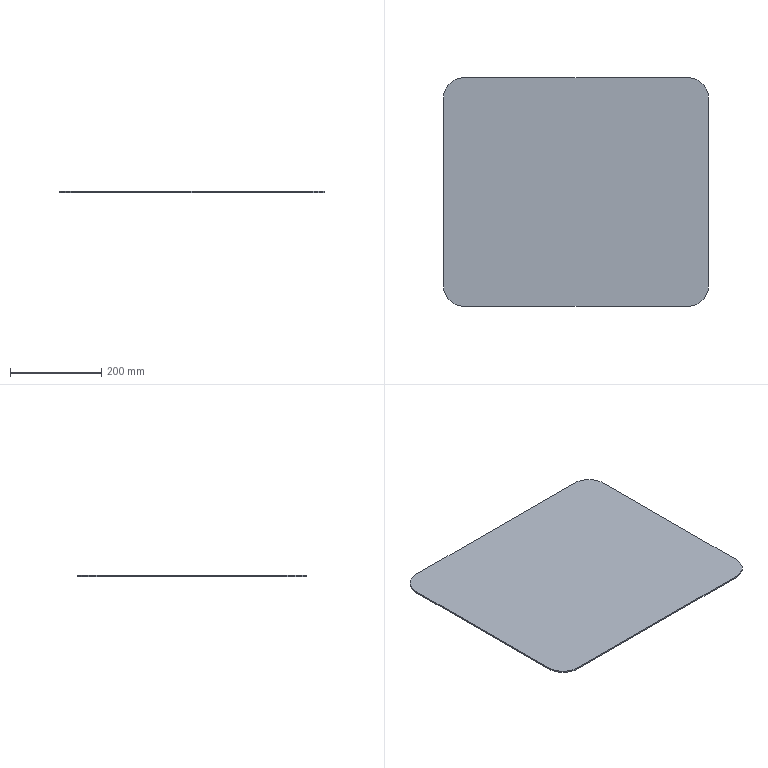Part | STEP file | Glass plate | 1 solid | 10 faces | box 580 x 500 x 3 mm | volume 864785 mm3 | plane 6 | cylinder 4 | commonest cylinder face diameters 90 x4
STEP:
#1=CARTESIAN_POINT('',(0.,0.,0.));
#2=DIRECTION('',(0.,0.,1.));
#3=DIRECTION('',(1.,0.,0.));
#4=AXIS2_PLACEMENT_3D('',#1,#2,#3);
#5=CARTESIAN_POINT('',(245.,-250.,0.));
#6=VERTEX_POINT('',#5);
#7=CARTESIAN_POINT('',(290.,-205.,0.));
#8=VERTEX_POINT('',#7);
#9=CARTESIAN_POINT('',(245.,-205.,0.));
#10=DIRECTION('',(0.,0.,1.));
#11=DIRECTION('',(1.,0.,0.));
#12=AXIS2_PLACEMENT_3D('',#9,#10,#11);
#13=CIRCLE('',#12,45.);
#14=CARTESIAN_POINT('',(0.,0.,0.));
#15=DIRECTION('',(0.,0.,1.));
#16=DIRECTION('',(1.,0.,0.));
#17=AXIS2_PLACEMENT_3D('',#14,#15,#16);
#18=PLANE('',#17);
#19=CARTESIAN_POINT('',(245.,-205.));
#20=DIRECTION('',(1.,0.));
#21=AXIS2_PLACEMENT_2D('',#19,#20);
#22=CIRCLE('',#21,45.);
#23=(GEOMETRIC_REPRESENTATION_CONTEXT(2)PARAMETRIC_REPRESENTATION_CONTEXT()REPRESENTATION_CONTEXT('',''));
#24=DEFINITIONAL_REPRESENTATION('',(#22),#23);
#25=PCURVE('',#18,#24);
#26=CARTESIAN_POINT('',(245.,-205.,-2.));
#27=DIRECTION('',(0.,0.,1.));
#28=DIRECTION('',(1.,0.,0.));
#29=AXIS2_PLACEMENT_3D('',#26,#27,#28);
#30=CYLINDRICAL_SURFACE('',#29,45.);
#31=CARTESIAN_POINT('',(0.,2.));
#32=DIRECTION('',(1.,0.));
#33=VECTOR('',#32,1.);
#34=LINE('',#31,#33);
#35=(GEOMETRIC_REPRESENTATION_CONTEXT(2)PARAMETRIC_REPRESENTATION_CONTEXT()REPRESENTATION_CONTEXT('',''));
#36=DEFINITIONAL_REPRESENTATION('',(#34),#35);
#37=PCURVE('',#30,#36);
#38=SURFACE_CURVE('',#13,(#25,#37),.PCURVE_S1.);
#39=EDGE_CURVE('',#6,#8,#38,.T.);
#40=ORIENTED_EDGE('',*,*,#39,.F.);
#41=CARTESIAN_POINT('',(-245.,-250.,0.));
#42=VERTEX_POINT('',#41);
#43=CARTESIAN_POINT('',(0.,-250.,0.));
#44=DIRECTION('',(1.,0.,0.));
#45=VECTOR('',#44,1.);
#46=LINE('',#43,#45);
#47=CARTESIAN_POINT('',(0.,-250.));
#48=DIRECTION('',(1.,0.));
#49=VECTOR('',#48,1.);
#50=LINE('',#47,#49);
#51=(GEOMETRIC_REPRESENTATION_CONTEXT(2)PARAMETRIC_REPRESENTATION_CONTEXT()REPRESENTATION_CONTEXT('',''));
#52=DEFINITIONAL_REPRESENTATION('',(#50),#51);
#53=PCURVE('',#18,#52);
#54=CARTESIAN_POINT('',(-245.,-250.,-2.));
#55=DIRECTION('',(0.,-1.,0.));
#56=DIRECTION('',(1.,0.,0.));
#57=AXIS2_PLACEMENT_3D('',#54,#55,#56);
#58=PLANE('',#57);
#59=CARTESIAN_POINT('',(245.,2.));
#60=DIRECTION('',(1.,0.));
#61=VECTOR('',#60,1.);
#62=LINE('',#59,#61);
#63=(GEOMETRIC_REPRESENTATION_CONTEXT(2)PARAMETRIC_REPRESENTATION_CONTEXT()REPRESENTATION_CONTEXT('',''));
#64=DEFINITIONAL_REPRESENTATION('',(#62),#63);
#65=PCURVE('',#58,#64);
#66=SURFACE_CURVE('',#46,(#53,#65),.PCURVE_S1.);
#67=EDGE_CURVE('',#42,#6,#66,.T.);
#68=ORIENTED_EDGE('',*,*,#67,.F.);
#69=CARTESIAN_POINT('',(-290.,-205.,0.));
#70=VERTEX_POINT('',#69);
#71=CARTESIAN_POINT('',(-245.,-205.,0.));
#72=DIRECTION('',(0.,0.,1.));
#73=DIRECTION('',(1.,0.,0.));
#74=AXIS2_PLACEMENT_3D('',#71,#72,#73);
#75=CIRCLE('',#74,45.);
#76=CARTESIAN_POINT('',(-245.,-205.));
#77=DIRECTION('',(1.,0.));
#78=AXIS2_PLACEMENT_2D('',#76,#77);
#79=CIRCLE('',#78,45.);
#80=(GEOMETRIC_REPRESENTATION_CONTEXT(2)PARAMETRIC_REPRESENTATION_CONTEXT()REPRESENTATION_CONTEXT('',''));
#81=DEFINITIONAL_REPRESENTATION('',(#79),#80);
#82=PCURVE('',#18,#81);
#83=CARTESIAN_POINT('',(-245.,-205.,-2.));
#84=DIRECTION('',(0.,0.,1.));
#85=DIRECTION('',(1.,0.,0.));
#86=AXIS2_PLACEMENT_3D('',#83,#84,#85);
#87=CYLINDRICAL_SURFACE('',#86,45.);
#88=CARTESIAN_POINT('',(0.,2.));
#89=DIRECTION('',(1.,0.));
#90=VECTOR('',#89,1.);
#91=LINE('',#88,#90);
#92=(GEOMETRIC_REPRESENTATION_CONTEXT(2)PARAMETRIC_REPRESENTATION_CONTEXT()REPRESENTATION_CONTEXT('',''));
#93=DEFINITIONAL_REPRESENTATION('',(#91),#92);
#94=PCURVE('',#87,#93);
#95=SURFACE_CURVE('',#75,(#82,#94),.PCURVE_S1.);
#96=EDGE_CURVE('',#70,#42,#95,.T.);
#97=ORIENTED_EDGE('',*,*,#96,.F.);
#98=CARTESIAN_POINT('',(-290.,205.,0.));
#99=VERTEX_POINT('',#98);
#100=CARTESIAN_POINT('',(-290.,0.,0.));
#101=DIRECTION('',(0.,-1.,0.));
#102=VECTOR('',#101,1.);
#103=LINE('',#100,#102);
#104=CARTESIAN_POINT('',(-290.,0.));
#105=DIRECTION('',(0.,-1.));
#106=VECTOR('',#105,1.);
#107=LINE('',#104,#106);
#108=(GEOMETRIC_REPRESENTATION_CONTEXT(2)PARAMETRIC_REPRESENTATION_CONTEXT()REPRESENTATION_CONTEXT('',''));
#109=DEFINITIONAL_REPRESENTATION('',(#107),#108);
#110=PCURVE('',#18,#109);
#111=CARTESIAN_POINT('',(-290.,205.,-2.));
#112=DIRECTION('',(-1.,0.,0.));
#113=DIRECTION('',(0.,-1.,0.));
#114=AXIS2_PLACEMENT_3D('',#111,#112,#113);
#115=PLANE('',#114);
#116=CARTESIAN_POINT('',(205.,2.));
#117=DIRECTION('',(1.,0.));
#118=VECTOR('',#117,1.);
#119=LINE('',#116,#118);
#120=(GEOMETRIC_REPRESENTATION_CONTEXT(2)PARAMETRIC_REPRESENTATION_CONTEXT()REPRESENTATION_CONTEXT('',''));
#121=DEFINITIONAL_REPRESENTATION('',(#119),#120);
#122=PCURVE('',#115,#121);
#123=SURFACE_CURVE('',#103,(#110,#122),.PCURVE_S1.);
#124=EDGE_CURVE('',#99,#70,#123,.T.);
#125=ORIENTED_EDGE('',*,*,#124,.F.);
#126=CARTESIAN_POINT('',(-245.,250.,0.));
#127=VERTEX_POINT('',#126);
#128=CARTESIAN_POINT('',(-245.,205.,0.));
#129=DIRECTION('',(0.,0.,1.));
#130=DIRECTION('',(1.,0.,0.));
#131=AXIS2_PLACEMENT_3D('',#128,#129,#130);
#132=CIRCLE('',#131,45.);
#133=CARTESIAN_POINT('',(-245.,205.));
#134=DIRECTION('',(1.,0.));
#135=AXIS2_PLACEMENT_2D('',#133,#134);
#136=CIRCLE('',#135,45.);
#137=(GEOMETRIC_REPRESENTATION_CONTEXT(2)PARAMETRIC_REPRESENTATION_CONTEXT()REPRESENTATION_CONTEXT('',''));
#138=DEFINITIONAL_REPRESENTATION('',(#136),#137);
#139=PCURVE('',#18,#138);
#140=CARTESIAN_POINT('',(-245.,205.,-2.));
#141=DIRECTION('',(0.,0.,1.));
#142=DIRECTION('',(1.,0.,0.));
#143=AXIS2_PLACEMENT_3D('',#140,#141,#142);
#144=CYLINDRICAL_SURFACE('',#143,45.);
#145=CARTESIAN_POINT('',(0.,2.));
#146=DIRECTION('',(1.,0.));
#147=VECTOR('',#146,1.);
#148=LINE('',#145,#147);
#149=(GEOMETRIC_REPRESENTATION_CONTEXT(2)PARAMETRIC_REPRESENTATION_CONTEXT()REPRESENTATION_CONTEXT('',''));
#150=DEFINITIONAL_REPRESENTATION('',(#148),#149);
#151=PCURVE('',#144,#150);
#152=SURFACE_CURVE('',#132,(#139,#151),.PCURVE_S1.);
#153=EDGE_CURVE('',#127,#99,#152,.T.);
#154=ORIENTED_EDGE('',*,*,#153,.F.);
#155=CARTESIAN_POINT('',(245.,250.,0.));
#156=VERTEX_POINT('',#155);
#157=CARTESIAN_POINT('',(0.,250.,0.));
#158=DIRECTION('',(-1.,0.,0.));
#159=VECTOR('',#158,1.);
#160=LINE('',#157,#159);
#161=CARTESIAN_POINT('',(0.,250.));
#162=DIRECTION('',(-1.,0.));
#163=VECTOR('',#162,1.);
#164=LINE('',#161,#163);
#165=(GEOMETRIC_REPRESENTATION_CONTEXT(2)PARAMETRIC_REPRESENTATION_CONTEXT()REPRESENTATION_CONTEXT('',''));
#166=DEFINITIONAL_REPRESENTATION('',(#164),#165);
#167=PCURVE('',#18,#166);
#168=CARTESIAN_POINT('',(245.,250.,-2.));
#169=DIRECTION('',(0.,1.,0.));
#170=DIRECTION('',(-1.,0.,0.));
#171=AXIS2_PLACEMENT_3D('',#168,#169,#170);
#172=PLANE('',#171);
#173=CARTESIAN_POINT('',(245.,2.));
#174=DIRECTION('',(1.,0.));
#175=VECTOR('',#174,1.);
#176=LINE('',#173,#175);
#177=(GEOMETRIC_REPRESENTATION_CONTEXT(2)PARAMETRIC_REPRESENTATION_CONTEXT()REPRESENTATION_CONTEXT('',''));
#178=DEFINITIONAL_REPRESENTATION('',(#176),#177);
#179=PCURVE('',#172,#178);
#180=SURFACE_CURVE('',#160,(#167,#179),.PCURVE_S1.);
#181=EDGE_CURVE('',#156,#127,#180,.T.);
#182=ORIENTED_EDGE('',*,*,#181,.F.);
#183=CARTESIAN_POINT('',(290.,205.,0.));
#184=VERTEX_POINT('',#183);
#185=CARTESIAN_POINT('',(245.,205.,0.));
#186=DIRECTION('',(0.,0.,1.));
#187=DIRECTION('',(1.,0.,0.));
#188=AXIS2_PLACEMENT_3D('',#185,#186,#187);
#189=CIRCLE('',#188,45.);
#190=CARTESIAN_POINT('',(245.,205.));
#191=DIRECTION('',(1.,0.));
#192=AXIS2_PLACEMENT_2D('',#190,#191);
#193=CIRCLE('',#192,45.);
#194=(GEOMETRIC_REPRESENTATION_CONTEXT(2)PARAMETRIC_REPRESENTATION_CONTEXT()REPRESENTATION_CONTEXT('',''));
#195=DEFINITIONAL_REPRESENTATION('',(#193),#194);
#196=PCURVE('',#18,#195);
#197=CARTESIAN_POINT('',(245.,205.,-2.));
#198=DIRECTION('',(0.,0.,1.));
#199=DIRECTION('',(1.,0.,0.));
#200=AXIS2_PLACEMENT_3D('',#197,#198,#199);
#201=CYLINDRICAL_SURFACE('',#200,45.);
#202=CARTESIAN_POINT('',(0.,2.));
#203=DIRECTION('',(1.,0.));
#204=VECTOR('',#203,1.);
#205=LINE('',#202,#204);
#206=(GEOMETRIC_REPRESENTATION_CONTEXT(2)PARAMETRIC_REPRESENTATION_CONTEXT()REPRESENTATION_CONTEXT('',''));
#207=DEFINITIONAL_REPRESENTATION('',(#205),#206);
#208=PCURVE('',#201,#207);
#209=SURFACE_CURVE('',#189,(#196,#208),.PCURVE_S1.);
#210=EDGE_CURVE('',#184,#156,#209,.T.);
#211=ORIENTED_EDGE('',*,*,#210,.F.);
#212=CARTESIAN_POINT('',(290.,0.,0.));
#213=DIRECTION('',(0.,1.,0.));
#214=VECTOR('',#213,1.);
#215=LINE('',#212,#214);
#216=CARTESIAN_POINT('',(290.,0.));
#217=DIRECTION('',(0.,1.));
#218=VECTOR('',#217,1.);
#219=LINE('',#216,#218);
#220=(GEOMETRIC_REPRESENTATION_CONTEXT(2)PARAMETRIC_REPRESENTATION_CONTEXT()REPRESENTATION_CONTEXT('',''));
#221=DEFINITIONAL_REPRESENTATION('',(#219),#220);
#222=PCURVE('',#18,#221);
#223=CARTESIAN_POINT('',(290.,-205.,-2.));
#224=DIRECTION('',(1.,0.,0.));
#225=DIRECTION('',(0.,1.,0.));
#226=AXIS2_PLACEMENT_3D('',#223,#224,#225);
#227=PLANE('',#226);
#228=CARTESIAN_POINT('',(205.,2.));
#229=DIRECTION('',(1.,0.));
#230=VECTOR('',#229,1.);
#231=LINE('',#228,#230);
#232=(GEOMETRIC_REPRESENTATION_CONTEXT(2)PARAMETRIC_REPRESENTATION_CONTEXT()REPRESENTATION_CONTEXT('',''));
#233=DEFINITIONAL_REPRESENTATION('',(#231),#232);
#234=PCURVE('',#227,#233);
#235=SURFACE_CURVE('',#215,(#222,#234),.PCURVE_S1.);
#236=EDGE_CURVE('',#8,#184,#235,.T.);
#237=ORIENTED_EDGE('',*,*,#236,.F.);
#238=EDGE_LOOP('',(#40,#68,#97,#125,#154,#182,#211,#237));
#239=FACE_BOUND('',#238,.T.);
#240=ADVANCED_FACE('',(#239),#18,.F.);
#241=ORIENTED_EDGE('',*,*,#39,.T.);
#242=CARTESIAN_POINT('',(290.,-205.,3.));
#243=VERTEX_POINT('',#242);
#244=CARTESIAN_POINT('',(290.,-205.,-2.));
#245=DIRECTION('',(0.,0.,1.));
#246=VECTOR('',#245,1.);
#247=LINE('',#244,#246);
#248=CARTESIAN_POINT('',(6.283,0.));
#249=DIRECTION('',(0.,1.));
#250=VECTOR('',#249,1.);
#251=LINE('',#248,#250);
#252=(GEOMETRIC_REPRESENTATION_CONTEXT(2)PARAMETRIC_REPRESENTATION_CONTEXT()REPRESENTATION_CONTEXT('',''));
#253=DEFINITIONAL_REPRESENTATION('',(#251),#252);
#254=PCURVE('',#30,#253);
#255=CARTESIAN_POINT('',(0.,0.));
#256=DIRECTION('',(0.,1.));
#257=VECTOR('',#256,1.);
#258=LINE('',#255,#257);
#259=(GEOMETRIC_REPRESENTATION_CONTEXT(2)PARAMETRIC_REPRESENTATION_CONTEXT()REPRESENTATION_CONTEXT('',''));
#260=DEFINITIONAL_REPRESENTATION('',(#258),#259);
#261=PCURVE('',#227,#260);
#262=SURFACE_CURVE('',#247,(#254,#261),.PCURVE_S1.);
#263=EDGE_CURVE('',#8,#243,#262,.T.);
#264=ORIENTED_EDGE('',*,*,#263,.T.);
#265=CARTESIAN_POINT('',(245.,-250.,3.));
#266=VERTEX_POINT('',#265);
#267=CARTESIAN_POINT('',(245.,-205.,3.));
#268=DIRECTION('',(0.,0.,1.));
#269=DIRECTION('',(1.,0.,0.));
#270=AXIS2_PLACEMENT_3D('',#267,#268,#269);
#271=CIRCLE('',#270,45.);
#272=CARTESIAN_POINT('',(0.,5.));
#273=DIRECTION('',(1.,0.));
#274=VECTOR('',#273,1.);
#275=LINE('',#272,#274);
#276=(GEOMETRIC_REPRESENTATION_CONTEXT(2)PARAMETRIC_REPRESENTATION_CONTEXT()REPRESENTATION_CONTEXT('',''));
#277=DEFINITIONAL_REPRESENTATION('',(#275),#276);
#278=PCURVE('',#30,#277);
#279=CARTESIAN_POINT('',(0.,0.,3.));
#280=DIRECTION('',(0.,0.,1.));
#281=DIRECTION('',(1.,0.,0.));
#282=AXIS2_PLACEMENT_3D('',#279,#280,#281);
#283=PLANE('',#282);
#284=CARTESIAN_POINT('',(245.,-205.));
#285=DIRECTION('',(1.,0.));
#286=AXIS2_PLACEMENT_2D('',#284,#285);
#287=CIRCLE('',#286,45.);
#288=(GEOMETRIC_REPRESENTATION_CONTEXT(2)PARAMETRIC_REPRESENTATION_CONTEXT()REPRESENTATION_CONTEXT('',''));
#289=DEFINITIONAL_REPRESENTATION('',(#287),#288);
#290=PCURVE('',#283,#289);
#291=SURFACE_CURVE('',#271,(#278,#290),.PCURVE_S1.);
#292=EDGE_CURVE('',#266,#243,#291,.T.);
#293=ORIENTED_EDGE('',*,*,#292,.F.);
#294=CARTESIAN_POINT('',(245.,-250.,-2.));
#295=DIRECTION('',(0.,0.,1.));
#296=VECTOR('',#295,1.);
#297=LINE('',#294,#296);
#298=CARTESIAN_POINT('',(4.712,0.));
#299=DIRECTION('',(0.,1.));
#300=VECTOR('',#299,1.);
#301=LINE('',#298,#300);
#302=(GEOMETRIC_REPRESENTATION_CONTEXT(2)PARAMETRIC_REPRESENTATION_CONTEXT()REPRESENTATION_CONTEXT('',''));
#303=DEFINITIONAL_REPRESENTATION('',(#301),#302);
#304=PCURVE('',#30,#303);
#305=CARTESIAN_POINT('',(490.,0.));
#306=DIRECTION('',(0.,1.));
#307=VECTOR('',#306,1.);
#308=LINE('',#305,#307);
#309=(GEOMETRIC_REPRESENTATION_CONTEXT(2)PARAMETRIC_REPRESENTATION_CONTEXT()REPRESENTATION_CONTEXT('',''));
#310=DEFINITIONAL_REPRESENTATION('',(#308),#309);
#311=PCURVE('',#58,#310);
#312=SURFACE_CURVE('',#297,(#304,#311),.PCURVE_S1.);
#313=EDGE_CURVE('',#6,#266,#312,.T.);
#314=ORIENTED_EDGE('',*,*,#313,.F.);
#315=EDGE_LOOP('',(#241,#264,#293,#314));
#316=FACE_BOUND('',#315,.T.);
#317=ADVANCED_FACE('',(#316),#30,.T.);
#318=ORIENTED_EDGE('',*,*,#67,.T.);
#319=ORIENTED_EDGE('',*,*,#313,.T.);
#320=CARTESIAN_POINT('',(-245.,-250.,3.));
#321=VERTEX_POINT('',#320);
#322=CARTESIAN_POINT('',(-245.,-250.,3.));
#323=DIRECTION('',(1.,0.,0.));
#324=VECTOR('',#323,1.);
#325=LINE('',#322,#324);
#326=CARTESIAN_POINT('',(0.,5.));
#327=DIRECTION('',(1.,0.));
#328=VECTOR('',#327,1.);
#329=LINE('',#326,#328);
#330=(GEOMETRIC_REPRESENTATION_CONTEXT(2)PARAMETRIC_REPRESENTATION_CONTEXT()REPRESENTATION_CONTEXT('',''));
#331=DEFINITIONAL_REPRESENTATION('',(#329),#330);
#332=PCURVE('',#58,#331);
#333=CARTESIAN_POINT('',(-245.,-250.));
#334=DIRECTION('',(1.,0.));
#335=VECTOR('',#334,1.);
#336=LINE('',#333,#335);
#337=(GEOMETRIC_REPRESENTATION_CONTEXT(2)PARAMETRIC_REPRESENTATION_CONTEXT()REPRESENTATION_CONTEXT('',''));
#338=DEFINITIONAL_REPRESENTATION('',(#336),#337);
#339=PCURVE('',#283,#338);
#340=SURFACE_CURVE('',#325,(#332,#339),.PCURVE_S1.);
#341=EDGE_CURVE('',#321,#266,#340,.T.);
#342=ORIENTED_EDGE('',*,*,#341,.F.);
#343=CARTESIAN_POINT('',(-245.,-250.,-2.));
#344=DIRECTION('',(0.,0.,1.));
#345=VECTOR('',#344,1.);
#346=LINE('',#343,#345);
#347=CARTESIAN_POINT('',(0.,0.));
#348=DIRECTION('',(0.,1.));
#349=VECTOR('',#348,1.);
#350=LINE('',#347,#349);
#351=(GEOMETRIC_REPRESENTATION_CONTEXT(2)PARAMETRIC_REPRESENTATION_CONTEXT()REPRESENTATION_CONTEXT('',''));
#352=DEFINITIONAL_REPRESENTATION('',(#350),#351);
#353=PCURVE('',#58,#352);
#354=CARTESIAN_POINT('',(4.712,0.));
#355=DIRECTION('',(0.,1.));
#356=VECTOR('',#355,1.);
#357=LINE('',#354,#356);
#358=(GEOMETRIC_REPRESENTATION_CONTEXT(2)PARAMETRIC_REPRESENTATION_CONTEXT()REPRESENTATION_CONTEXT('',''));
#359=DEFINITIONAL_REPRESENTATION('',(#357),#358);
#360=PCURVE('',#87,#359);
#361=SURFACE_CURVE('',#346,(#353,#360),.PCURVE_S1.);
#362=EDGE_CURVE('',#42,#321,#361,.T.);
#363=ORIENTED_EDGE('',*,*,#362,.F.);
#364=EDGE_LOOP('',(#318,#319,#342,#363));
#365=FACE_BOUND('',#364,.T.);
#366=ADVANCED_FACE('',(#365),#58,.T.);
#367=ORIENTED_EDGE('',*,*,#96,.T.);
#368=ORIENTED_EDGE('',*,*,#362,.T.);
#369=CARTESIAN_POINT('',(-290.,-205.,3.));
#370=VERTEX_POINT('',#369);
#371=CARTESIAN_POINT('',(-245.,-205.,3.));
#372=DIRECTION('',(0.,0.,1.));
#373=DIRECTION('',(1.,0.,0.));
#374=AXIS2_PLACEMENT_3D('',#371,#372,#373);
#375=CIRCLE('',#374,45.);
#376=CARTESIAN_POINT('',(0.,5.));
#377=DIRECTION('',(1.,0.));
#378=VECTOR('',#377,1.);
#379=LINE('',#376,#378);
#380=(GEOMETRIC_REPRESENTATION_CONTEXT(2)PARAMETRIC_REPRESENTATION_CONTEXT()REPRESENTATION_CONTEXT('',''));
#381=DEFINITIONAL_REPRESENTATION('',(#379),#380);
#382=PCURVE('',#87,#381);
#383=CARTESIAN_POINT('',(-245.,-205.));
#384=DIRECTION('',(1.,0.));
#385=AXIS2_PLACEMENT_2D('',#383,#384);
#386=CIRCLE('',#385,45.);
#387=(GEOMETRIC_REPRESENTATION_CONTEXT(2)PARAMETRIC_REPRESENTATION_CONTEXT()REPRESENTATION_CONTEXT('',''));
#388=DEFINITIONAL_REPRESENTATION('',(#386),#387);
#389=PCURVE('',#283,#388);
#390=SURFACE_CURVE('',#375,(#382,#389),.PCURVE_S1.);
#391=EDGE_CURVE('',#370,#321,#390,.T.);
#392=ORIENTED_EDGE('',*,*,#391,.F.);
#393=CARTESIAN_POINT('',(-290.,-205.,-2.));
#394=DIRECTION('',(0.,0.,1.));
#395=VECTOR('',#394,1.);
#396=LINE('',#393,#395);
#397=CARTESIAN_POINT('',(3.142,0.));
#398=DIRECTION('',(0.,1.));
#399=VECTOR('',#398,1.);
#400=LINE('',#397,#399);
#401=(GEOMETRIC_REPRESENTATION_CONTEXT(2)PARAMETRIC_REPRESENTATION_CONTEXT()REPRESENTATION_CONTEXT('',''));
#402=DEFINITIONAL_REPRESENTATION('',(#400),#401);
#403=PCURVE('',#87,#402);
#404=CARTESIAN_POINT('',(410.,0.));
#405=DIRECTION('',(0.,1.));
#406=VECTOR('',#405,1.);
#407=LINE('',#404,#406);
#408=(GEOMETRIC_REPRESENTATION_CONTEXT(2)PARAMETRIC_REPRESENTATION_CONTEXT()REPRESENTATION_CONTEXT('',''));
#409=DEFINITIONAL_REPRESENTATION('',(#407),#408);
#410=PCURVE('',#115,#409);
#411=SURFACE_CURVE('',#396,(#403,#410),.PCURVE_S1.);
#412=EDGE_CURVE('',#70,#370,#411,.T.);
#413=ORIENTED_EDGE('',*,*,#412,.F.);
#414=EDGE_LOOP('',(#367,#368,#392,#413));
#415=FACE_BOUND('',#414,.T.);
#416=ADVANCED_FACE('',(#415),#87,.T.);
#417=ORIENTED_EDGE('',*,*,#124,.T.);
#418=ORIENTED_EDGE('',*,*,#412,.T.);
#419=CARTESIAN_POINT('',(-290.,205.,3.));
#420=VERTEX_POINT('',#419);
#421=CARTESIAN_POINT('',(-290.,205.,3.));
#422=DIRECTION('',(0.,-1.,0.));
#423=VECTOR('',#422,1.);
#424=LINE('',#421,#423);
#425=CARTESIAN_POINT('',(0.,5.));
#426=DIRECTION('',(1.,0.));
#427=VECTOR('',#426,1.);
#428=LINE('',#425,#427);
#429=(GEOMETRIC_REPRESENTATION_CONTEXT(2)PARAMETRIC_REPRESENTATION_CONTEXT()REPRESENTATION_CONTEXT('',''));
#430=DEFINITIONAL_REPRESENTATION('',(#428),#429);
#431=PCURVE('',#115,#430);
#432=CARTESIAN_POINT('',(-290.,205.));
#433=DIRECTION('',(0.,-1.));
#434=VECTOR('',#433,1.);
#435=LINE('',#432,#434);
#436=(GEOMETRIC_REPRESENTATION_CONTEXT(2)PARAMETRIC_REPRESENTATION_CONTEXT()REPRESENTATION_CONTEXT('',''));
#437=DEFINITIONAL_REPRESENTATION('',(#435),#436);
#438=PCURVE('',#283,#437);
#439=SURFACE_CURVE('',#424,(#431,#438),.PCURVE_S1.);
#440=EDGE_CURVE('',#420,#370,#439,.T.);
#441=ORIENTED_EDGE('',*,*,#440,.F.);
#442=CARTESIAN_POINT('',(-290.,205.,-2.));
#443=DIRECTION('',(0.,0.,1.));
#444=VECTOR('',#443,1.);
#445=LINE('',#442,#444);
#446=CARTESIAN_POINT('',(0.,0.));
#447=DIRECTION('',(0.,1.));
#448=VECTOR('',#447,1.);
#449=LINE('',#446,#448);
#450=(GEOMETRIC_REPRESENTATION_CONTEXT(2)PARAMETRIC_REPRESENTATION_CONTEXT()REPRESENTATION_CONTEXT('',''));
#451=DEFINITIONAL_REPRESENTATION('',(#449),#450);
#452=PCURVE('',#115,#451);
#453=CARTESIAN_POINT('',(3.142,0.));
#454=DIRECTION('',(0.,1.));
#455=VECTOR('',#454,1.);
#456=LINE('',#453,#455);
#457=(GEOMETRIC_REPRESENTATION_CONTEXT(2)PARAMETRIC_REPRESENTATION_CONTEXT()REPRESENTATION_CONTEXT('',''));
#458=DEFINITIONAL_REPRESENTATION('',(#456),#457);
#459=PCURVE('',#144,#458);
#460=SURFACE_CURVE('',#445,(#452,#459),.PCURVE_S1.);
#461=EDGE_CURVE('',#99,#420,#460,.T.);
#462=ORIENTED_EDGE('',*,*,#461,.F.);
#463=EDGE_LOOP('',(#417,#418,#441,#462));
#464=FACE_BOUND('',#463,.T.);
#465=ADVANCED_FACE('',(#464),#115,.T.);
#466=ORIENTED_EDGE('',*,*,#153,.T.);
#467=ORIENTED_EDGE('',*,*,#461,.T.);
#468=CARTESIAN_POINT('',(-245.,250.,3.));
#469=VERTEX_POINT('',#468);
#470=CARTESIAN_POINT('',(-245.,205.,3.));
#471=DIRECTION('',(0.,0.,1.));
#472=DIRECTION('',(1.,0.,0.));
#473=AXIS2_PLACEMENT_3D('',#470,#471,#472);
#474=CIRCLE('',#473,45.);
#475=CARTESIAN_POINT('',(0.,5.));
#476=DIRECTION('',(1.,0.));
#477=VECTOR('',#476,1.);
#478=LINE('',#475,#477);
#479=(GEOMETRIC_REPRESENTATION_CONTEXT(2)PARAMETRIC_REPRESENTATION_CONTEXT()REPRESENTATION_CONTEXT('',''));
#480=DEFINITIONAL_REPRESENTATION('',(#478),#479);
#481=PCURVE('',#144,#480);
#482=CARTESIAN_POINT('',(-245.,205.));
#483=DIRECTION('',(1.,0.));
#484=AXIS2_PLACEMENT_2D('',#482,#483);
#485=CIRCLE('',#484,45.);
#486=(GEOMETRIC_REPRESENTATION_CONTEXT(2)PARAMETRIC_REPRESENTATION_CONTEXT()REPRESENTATION_CONTEXT('',''));
#487=DEFINITIONAL_REPRESENTATION('',(#485),#486);
#488=PCURVE('',#283,#487);
#489=SURFACE_CURVE('',#474,(#481,#488),.PCURVE_S1.);
#490=EDGE_CURVE('',#469,#420,#489,.T.);
#491=ORIENTED_EDGE('',*,*,#490,.F.);
#492=CARTESIAN_POINT('',(-245.,250.,-2.));
#493=DIRECTION('',(0.,0.,1.));
#494=VECTOR('',#493,1.);
#495=LINE('',#492,#494);
#496=CARTESIAN_POINT('',(1.571,0.));
#497=DIRECTION('',(0.,1.));
#498=VECTOR('',#497,1.);
#499=LINE('',#496,#498);
#500=(GEOMETRIC_REPRESENTATION_CONTEXT(2)PARAMETRIC_REPRESENTATION_CONTEXT()REPRESENTATION_CONTEXT('',''));
#501=DEFINITIONAL_REPRESENTATION('',(#499),#500);
#502=PCURVE('',#144,#501);
#503=CARTESIAN_POINT('',(490.,0.));
#504=DIRECTION('',(0.,1.));
#505=VECTOR('',#504,1.);
#506=LINE('',#503,#505);
#507=(GEOMETRIC_REPRESENTATION_CONTEXT(2)PARAMETRIC_REPRESENTATION_CONTEXT()REPRESENTATION_CONTEXT('',''));
#508=DEFINITIONAL_REPRESENTATION('',(#506),#507);
#509=PCURVE('',#172,#508);
#510=SURFACE_CURVE('',#495,(#502,#509),.PCURVE_S1.);
#511=EDGE_CURVE('',#127,#469,#510,.T.);
#512=ORIENTED_EDGE('',*,*,#511,.F.);
#513=EDGE_LOOP('',(#466,#467,#491,#512));
#514=FACE_BOUND('',#513,.T.);
#515=ADVANCED_FACE('',(#514),#144,.T.);
#516=ORIENTED_EDGE('',*,*,#181,.T.);
#517=ORIENTED_EDGE('',*,*,#511,.T.);
#518=CARTESIAN_POINT('',(245.,250.,3.));
#519=VERTEX_POINT('',#518);
#520=CARTESIAN_POINT('',(245.,250.,3.));
#521=DIRECTION('',(-1.,0.,0.));
#522=VECTOR('',#521,1.);
#523=LINE('',#520,#522);
#524=CARTESIAN_POINT('',(0.,5.));
#525=DIRECTION('',(1.,0.));
#526=VECTOR('',#525,1.);
#527=LINE('',#524,#526);
#528=(GEOMETRIC_REPRESENTATION_CONTEXT(2)PARAMETRIC_REPRESENTATION_CONTEXT()REPRESENTATION_CONTEXT('',''));
#529=DEFINITIONAL_REPRESENTATION('',(#527),#528);
#530=PCURVE('',#172,#529);
#531=CARTESIAN_POINT('',(245.,250.));
#532=DIRECTION('',(-1.,0.));
#533=VECTOR('',#532,1.);
#534=LINE('',#531,#533);
#535=(GEOMETRIC_REPRESENTATION_CONTEXT(2)PARAMETRIC_REPRESENTATION_CONTEXT()REPRESENTATION_CONTEXT('',''));
#536=DEFINITIONAL_REPRESENTATION('',(#534),#535);
#537=PCURVE('',#283,#536);
#538=SURFACE_CURVE('',#523,(#530,#537),.PCURVE_S1.);
#539=EDGE_CURVE('',#519,#469,#538,.T.);
#540=ORIENTED_EDGE('',*,*,#539,.F.);
#541=CARTESIAN_POINT('',(245.,250.,-2.));
#542=DIRECTION('',(0.,0.,1.));
#543=VECTOR('',#542,1.);
#544=LINE('',#541,#543);
#545=CARTESIAN_POINT('',(0.,0.));
#546=DIRECTION('',(0.,1.));
#547=VECTOR('',#546,1.);
#548=LINE('',#545,#547);
#549=(GEOMETRIC_REPRESENTATION_CONTEXT(2)PARAMETRIC_REPRESENTATION_CONTEXT()REPRESENTATION_CONTEXT('',''));
#550=DEFINITIONAL_REPRESENTATION('',(#548),#549);
#551=PCURVE('',#172,#550);
#552=CARTESIAN_POINT('',(1.571,0.));
#553=DIRECTION('',(0.,1.));
#554=VECTOR('',#553,1.);
#555=LINE('',#552,#554);
#556=(GEOMETRIC_REPRESENTATION_CONTEXT(2)PARAMETRIC_REPRESENTATION_CONTEXT()REPRESENTATION_CONTEXT('',''));
#557=DEFINITIONAL_REPRESENTATION('',(#555),#556);
#558=PCURVE('',#201,#557);
#559=SURFACE_CURVE('',#544,(#551,#558),.PCURVE_S1.);
#560=EDGE_CURVE('',#156,#519,#559,.T.);
#561=ORIENTED_EDGE('',*,*,#560,.F.);
#562=EDGE_LOOP('',(#516,#517,#540,#561));
#563=FACE_BOUND('',#562,.T.);
#564=ADVANCED_FACE('',(#563),#172,.T.);
#565=ORIENTED_EDGE('',*,*,#210,.T.);
#566=ORIENTED_EDGE('',*,*,#560,.T.);
#567=CARTESIAN_POINT('',(290.,205.,3.));
#568=VERTEX_POINT('',#567);
#569=CARTESIAN_POINT('',(245.,205.,3.));
#570=DIRECTION('',(0.,0.,1.));
#571=DIRECTION('',(1.,0.,0.));
#572=AXIS2_PLACEMENT_3D('',#569,#570,#571);
#573=CIRCLE('',#572,45.);
#574=CARTESIAN_POINT('',(0.,5.));
#575=DIRECTION('',(1.,0.));
#576=VECTOR('',#575,1.);
#577=LINE('',#574,#576);
#578=(GEOMETRIC_REPRESENTATION_CONTEXT(2)PARAMETRIC_REPRESENTATION_CONTEXT()REPRESENTATION_CONTEXT('',''));
#579=DEFINITIONAL_REPRESENTATION('',(#577),#578);
#580=PCURVE('',#201,#579);
#581=CARTESIAN_POINT('',(245.,205.));
#582=DIRECTION('',(1.,0.));
#583=AXIS2_PLACEMENT_2D('',#581,#582);
#584=CIRCLE('',#583,45.);
#585=(GEOMETRIC_REPRESENTATION_CONTEXT(2)PARAMETRIC_REPRESENTATION_CONTEXT()REPRESENTATION_CONTEXT('',''));
#586=DEFINITIONAL_REPRESENTATION('',(#584),#585);
#587=PCURVE('',#283,#586);
#588=SURFACE_CURVE('',#573,(#580,#587),.PCURVE_S1.);
#589=EDGE_CURVE('',#568,#519,#588,.T.);
#590=ORIENTED_EDGE('',*,*,#589,.F.);
#591=CARTESIAN_POINT('',(290.,205.,-2.));
#592=DIRECTION('',(0.,0.,1.));
#593=VECTOR('',#592,1.);
#594=LINE('',#591,#593);
#595=CARTESIAN_POINT('',(0.,0.));
#596=DIRECTION('',(0.,1.));
#597=VECTOR('',#596,1.);
#598=LINE('',#595,#597);
#599=(GEOMETRIC_REPRESENTATION_CONTEXT(2)PARAMETRIC_REPRESENTATION_CONTEXT()REPRESENTATION_CONTEXT('',''));
#600=DEFINITIONAL_REPRESENTATION('',(#598),#599);
#601=PCURVE('',#201,#600);
#602=CARTESIAN_POINT('',(410.,0.));
#603=DIRECTION('',(0.,1.));
#604=VECTOR('',#603,1.);
#605=LINE('',#602,#604);
#606=(GEOMETRIC_REPRESENTATION_CONTEXT(2)PARAMETRIC_REPRESENTATION_CONTEXT()REPRESENTATION_CONTEXT('',''));
#607=DEFINITIONAL_REPRESENTATION('',(#605),#606);
#608=PCURVE('',#227,#607);
#609=SURFACE_CURVE('',#594,(#601,#608),.PCURVE_S1.);
#610=EDGE_CURVE('',#184,#568,#609,.T.);
#611=ORIENTED_EDGE('',*,*,#610,.F.);
#612=EDGE_LOOP('',(#565,#566,#590,#611));
#613=FACE_BOUND('',#612,.T.);
#614=ADVANCED_FACE('',(#613),#201,.T.);
#615=ORIENTED_EDGE('',*,*,#236,.T.);
#616=ORIENTED_EDGE('',*,*,#610,.T.);
#617=CARTESIAN_POINT('',(290.,-205.,3.));
#618=DIRECTION('',(0.,1.,0.));
#619=VECTOR('',#618,1.);
#620=LINE('',#617,#619);
#621=CARTESIAN_POINT('',(0.,5.));
#622=DIRECTION('',(1.,0.));
#623=VECTOR('',#622,1.);
#624=LINE('',#621,#623);
#625=(GEOMETRIC_REPRESENTATION_CONTEXT(2)PARAMETRIC_REPRESENTATION_CONTEXT()REPRESENTATION_CONTEXT('',''));
#626=DEFINITIONAL_REPRESENTATION('',(#624),#625);
#627=PCURVE('',#227,#626);
#628=CARTESIAN_POINT('',(290.,-205.));
#629=DIRECTION('',(0.,1.));
#630=VECTOR('',#629,1.);
#631=LINE('',#628,#630);
#632=(GEOMETRIC_REPRESENTATION_CONTEXT(2)PARAMETRIC_REPRESENTATION_CONTEXT()REPRESENTATION_CONTEXT('',''));
#633=DEFINITIONAL_REPRESENTATION('',(#631),#632);
#634=PCURVE('',#283,#633);
#635=SURFACE_CURVE('',#620,(#627,#634),.PCURVE_S1.);
#636=EDGE_CURVE('',#243,#568,#635,.T.);
#637=ORIENTED_EDGE('',*,*,#636,.F.);
#638=ORIENTED_EDGE('',*,*,#263,.F.);
#639=EDGE_LOOP('',(#615,#616,#637,#638));
#640=FACE_BOUND('',#639,.T.);
#641=ADVANCED_FACE('',(#640),#227,.T.);
#642=ORIENTED_EDGE('',*,*,#341,.T.);
#643=ORIENTED_EDGE('',*,*,#292,.T.);
#644=ORIENTED_EDGE('',*,*,#636,.T.);
#645=ORIENTED_EDGE('',*,*,#589,.T.);
#646=ORIENTED_EDGE('',*,*,#539,.T.);
#647=ORIENTED_EDGE('',*,*,#490,.T.);
#648=ORIENTED_EDGE('',*,*,#440,.T.);
#649=ORIENTED_EDGE('',*,*,#391,.T.);
#650=EDGE_LOOP('',(#642,#643,#644,#645,#646,#647,#648,#649));
#651=FACE_BOUND('',#650,.T.);
#652=ADVANCED_FACE('',(#651),#283,.T.);
#653=CLOSED_SHELL('',(#240,#317,#366,#416,#465,#515,#564,#614,#641,#652));
#654=MANIFOLD_SOLID_BREP('',#653);
#655=(LENGTH_UNIT()NAMED_UNIT(*)SI_UNIT(.MILLI.,.METRE.));
#656=UNCERTAINTY_MEASURE_WITH_UNIT(LENGTH_MEASURE(0.0000001),#655,'','');
#657=(NAMED_UNIT(*)PLANE_ANGLE_UNIT()SI_UNIT($,.RADIAN.));
#658=(NAMED_UNIT(*)SI_UNIT($,.STERADIAN.)SOLID_ANGLE_UNIT());
#659=(GEOMETRIC_REPRESENTATION_CONTEXT(3)GLOBAL_UNCERTAINTY_ASSIGNED_CONTEXT((#656))GLOBAL_UNIT_ASSIGNED_CONTEXT((#655,#657,#658))REPRESENTATION_CONTEXT('',''));
#660=ADVANCED_BREP_SHAPE_REPRESENTATION('',(#4,#654),#659);